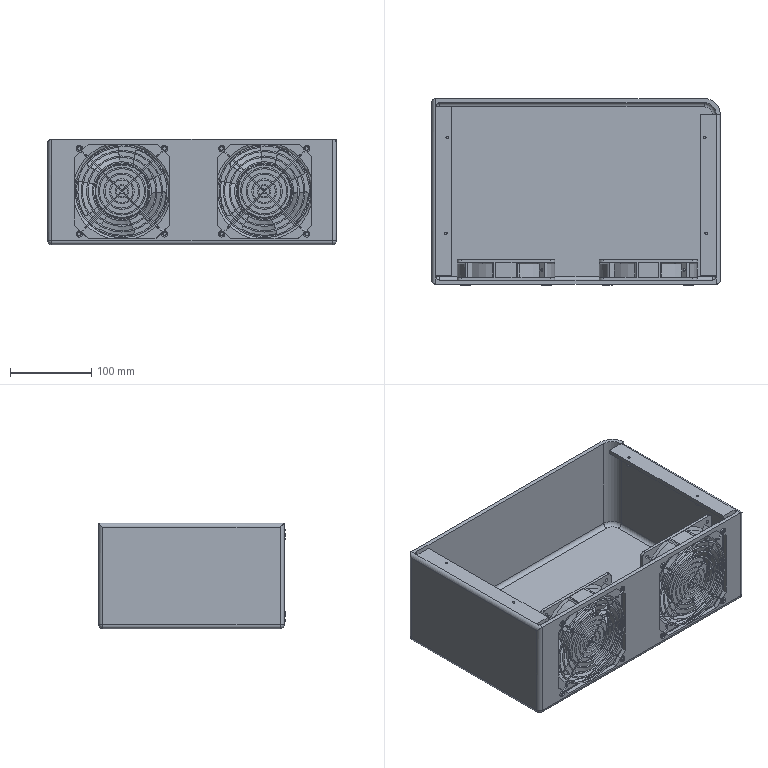Part | NX | features BREP 1 | 25 solids | 607 faces | box 355 x 229.658 x 130 mm | volume 1267062 mm3 | plane 293 | cylinder 124 | spline 82 | torus 70 | cone 32 | sphere 6 | commonest cylinder face diameters 10 x34 4.2 x24 120 x14 4 x12 1.6 x8 1.8 x6